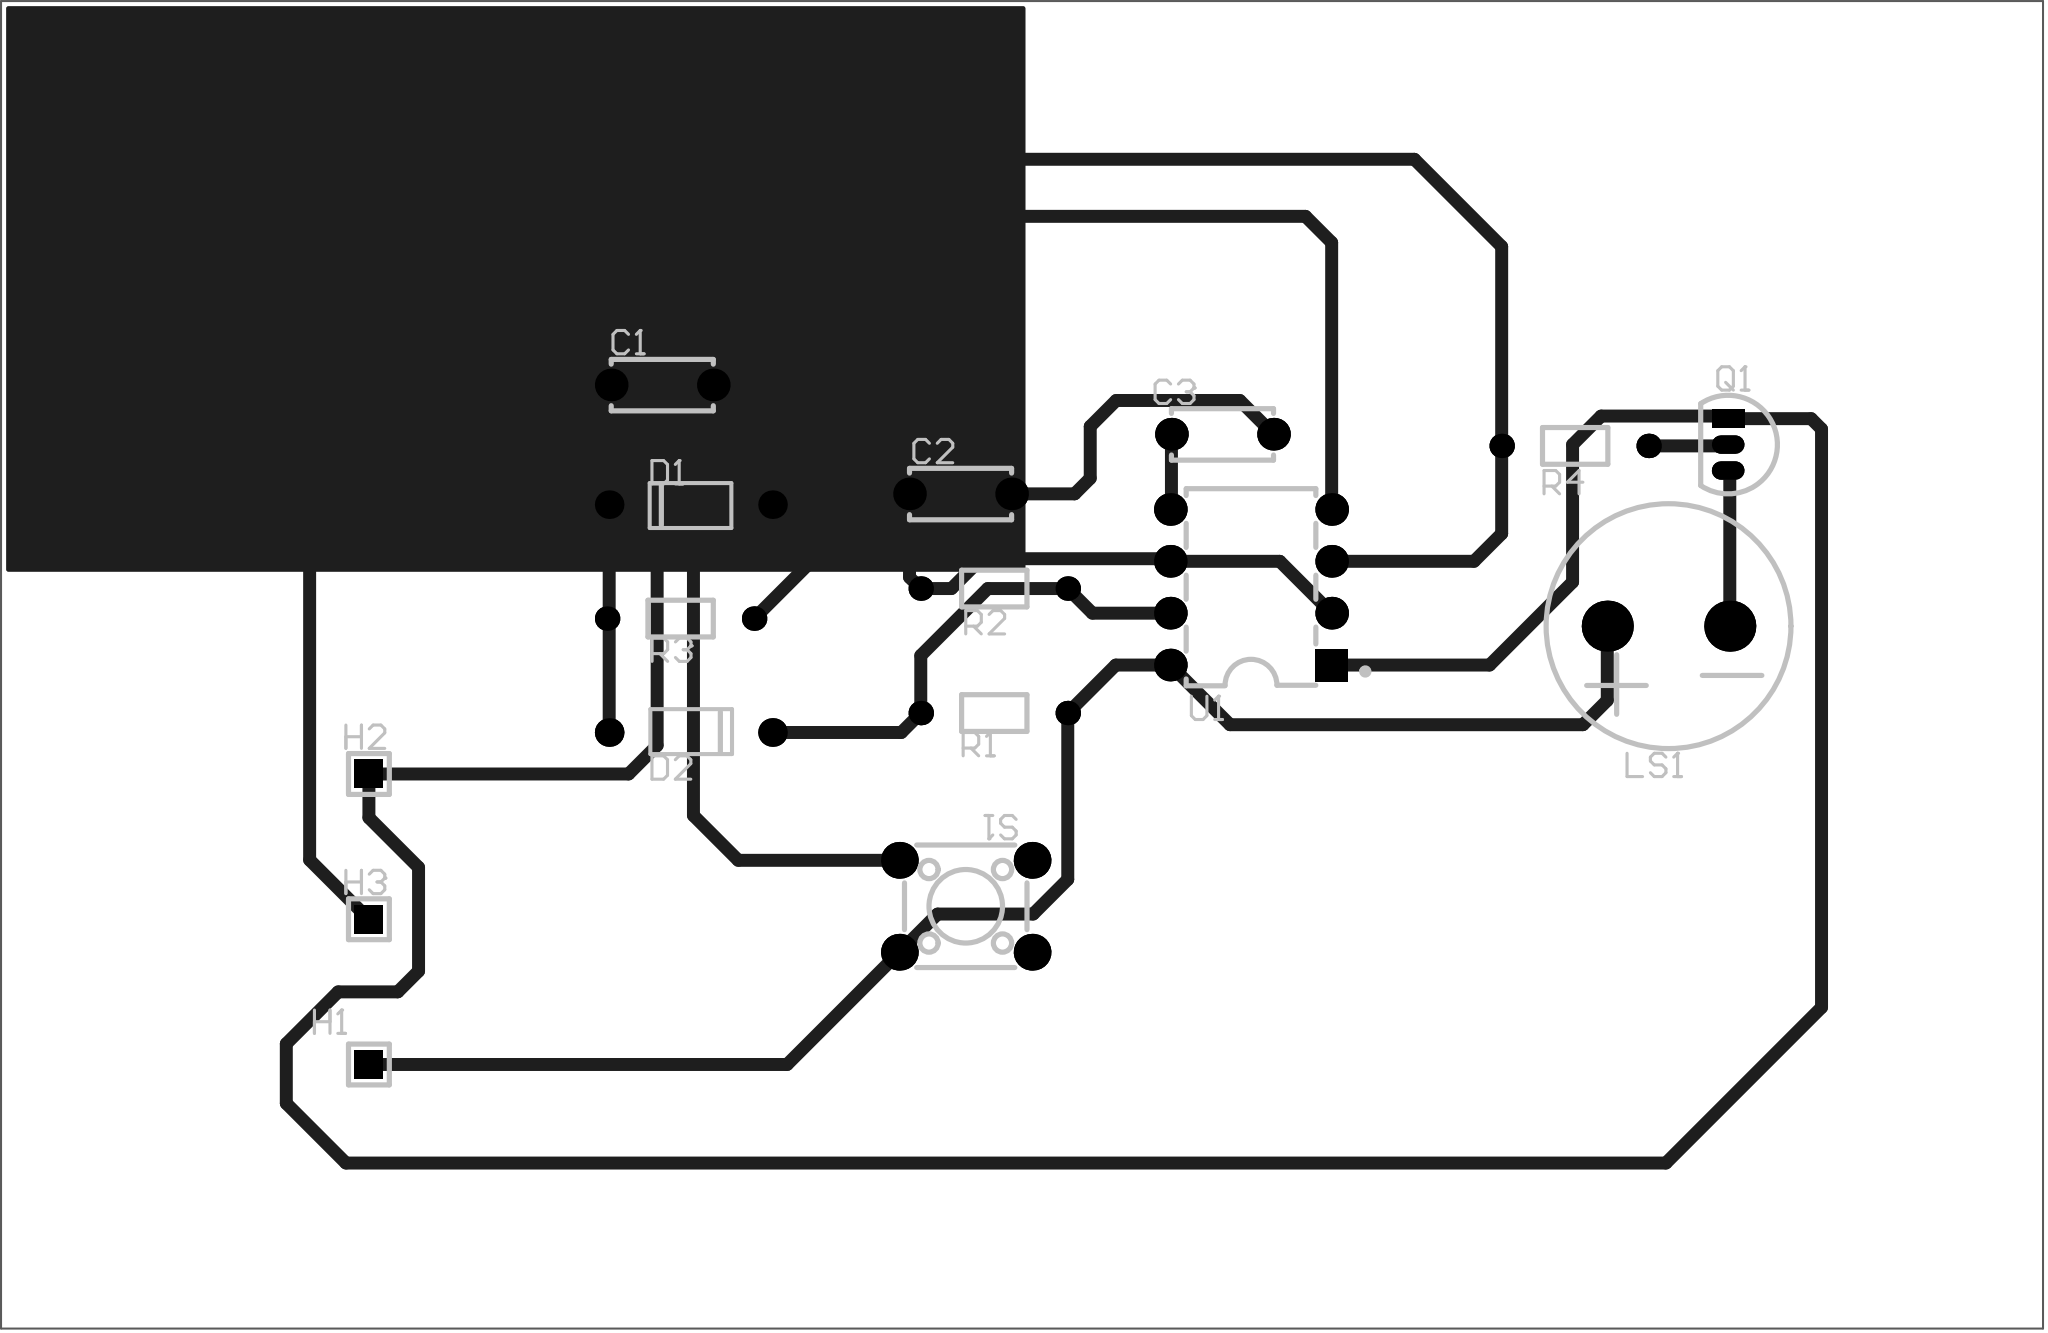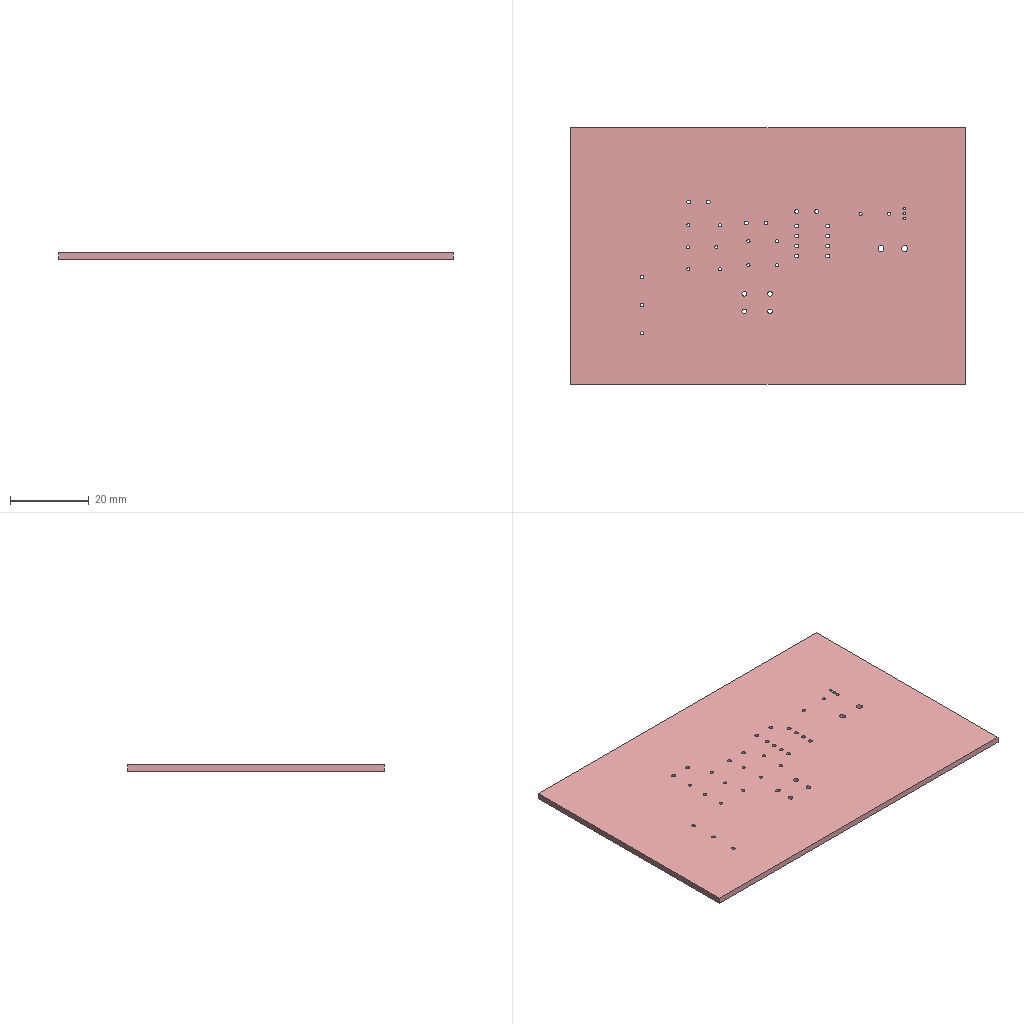Circuit board layout | Altium Designer | box 100 x 65 x 1.6 mm
Layer stack:
# Altium Designer layer stack of  (unit mm; dielectric type: 0 none, 1 core, 2 prepreg, 3 surface material)
index,name,kind,layer,copper_thickness_mm,dielectric_type,dielectric_thickness_mm,dielectric_material,dielectric_constant
0,Top Paste Mask Layer,other,,,,,,
1,Top Silkscreen Layer,other,,,,,,
2,Top Solder Mask Layer,dielectric,,,3,0.01,,3.3
3,Top Layer,copper,Top Layer,0.035,,,,
4,Dielectric1,dielectric,,,3,1.51,FR4,4.5
5,Bottom Layer,copper,Bottom Layer,0.035,,,,
6,Bottom Solder Mask Layer,dielectric,,,3,0.01,,3.3
7,Bottom Silkscreen Layer,other,,,,,,
8,Bottom Paste Mask Layer,other,,,,,,
# drill layer pairs: low layer,high layer
drill_pair,Top Layer,Bottom Layer
Part placement:
Designator,Comment,Layer,Footprint,Center-X(mm),Center-Y(mm),Rotation
LS1,buzzer,TopLayer,BUZ-TH_BD12.0-P6.00-D0.9-RD,163.068,110.593,180
D1,1N4148,TopLayer,DO-35_BD2.2-L4.0-D0.50_1N4148,115.189,116.541,180
D2,1N4148,TopLayer,DO-35_BD2.2-L4.0-D0.50_1N4148,115.189,105.386,0
Q1,,TopLayer,S8050_TO_92,165.989,119.483,270
R3,10kΩ,TopLayer,Res_1/8W,114.688,110.964,180
R2,5kΩ,TopLayer,Res_1/8W,130.048,112.434,0
R1,10kΩ,TopLayer,Res_1/8W,130.048,106.338,0
R4,120Ω,TopLayer,Res_1/8W,158.496,119.419,0
S1,,TopLayer,SW-TH_4P-L6.0-W6.0-P4.50-LS6.5,128.651,96.877,0
U1,LM555CM,TopLayer,PDIP-8_L9.6-W6.4-P2.54-LS7.9-BL-1,142.621,112.498,90
C1,100nF,TopLayer,CAP-TH_L5.0-W2.5-P5.00-D1.0,113.789,122.404,0
C2,0.1uF,TopLayer,CAP-TH_L5.0-W2.5-P5.00-D1.0,128.397,117.07,0
C3,0.01uF,TopLayer,CAP-TH_L5.0-W2.5-P5.00-D1.0,141.224,119.991,0
H1,,TopLayer,HDR-TH_1P-V-M_XKB_X4611WV-01I-C28D40,99.422,89.13,0
H2,,TopLayer,HDR-TH_1P-V-M_XKB_X4611WV-01I-C28D40,99.422,103.354,0
H3,,TopLayer,HDR-TH_1P-V-M_XKB_X4611WV-01I-C28D40,99.422,96.242,0
Pad and via stacks:
# Altium Designer via and pad stacks of  (unit mm). Each distinct definition once, with the count of objects using it.
# via: kind,start_layer,end_layer,hole_mm,diameter_mm,mode(0 simple;1 top-mid-bottom;2 full stack),diameter_per_layer,count,example_net
# pad: kind,layer,hole_mm,hole_type(0 round;1 square;2 slot),plating,top_size,top_shape(1 round;2 rect;3 octagon;9 rounded rect),mid_size,bottom_size,mode,footprint,size_per_layer,count,example
pad,Multi-Layer,1.5,0,plated,2.5x2.5,1,2.5x2.5,2.5x2.5,0,BUZ-TH_BD12.0-P6.00-D0.9-RD,,2,LS1.1
pad,Multi-Layer,0.8,0,plated,1.4x1.4,1,1.4x1.4,1.4x1.4,0,DO-35_BD2.2-L4.0-D0.50_1N4148,,4,D1.2
pad,Multi-Layer,0.701,0,plated,0.8992x1.6,2,0.8992x1.6,0.8992x1.6,0,S8050_TO_92,,1,Q1.1
pad,Multi-Layer,0.701,0,plated,0.8992x1.6,1,0.8992x1.6,0.8992x1.6,0,S8050_TO_92,,2,Q1.2
pad,Multi-Layer,0.8001,0,plated,1.199x1.199,1,1.199x1.199,1.199x1.199,0,Res_1/8W,,8,R3.1
pad,Multi-Layer,1.2,0,plated,1.8x1.8,1,1.8x1.8,1.8x1.8,0,SW-TH_4P-L6.0-W6.0-P4.50-LS6.5,,4,S1.1
pad,Multi-Layer,1,0,plated,1.6x1.6,1,1.6x1.6,1.6x1.6,0,PDIP-8_L9.6-W6.4-P2.54-LS7.9-BL-1,,7,U1.8
pad,Multi-Layer,1,0,plated,1.6x1.6,2,1.6x1.6,1.6x1.6,0,PDIP-8_L9.6-W6.4-P2.54-LS7.9-BL-1,,1,U1.1
pad,Multi-Layer,1,0,plated,1.6x1.6,1,1.6x1.6,1.6x1.6,0,CAP-TH_L5.0-W2.5-P5.00-D1.0,,6,C1.1
pad,Multi-Layer,0.9,0,plated,1.4x1.4,2,1.4x1.4,1.4x1.4,0,HDR-TH_1P-V-M_XKB_X4611WV-01I-C28D40,,3,H1.1
Copper pours:
name,layer,net,type(0 solid;1 hatched;2 none)
Top Layer-GND,Top Layer,GND,0
Bottom Layer-GND,Bottom Layer,GND,0
Design rules, without the lines most boards share:
# Altium Designer design rules of  (exported by Altium Designer, unit mm)
# columns: name | kind | enabled | priority | scope1 | scope2 | descriptor | typed fields (field=value)
creepage | 65 | enabled | 1 | All | All | Creepage Distance Constraint =(0mil) (All),(All) |